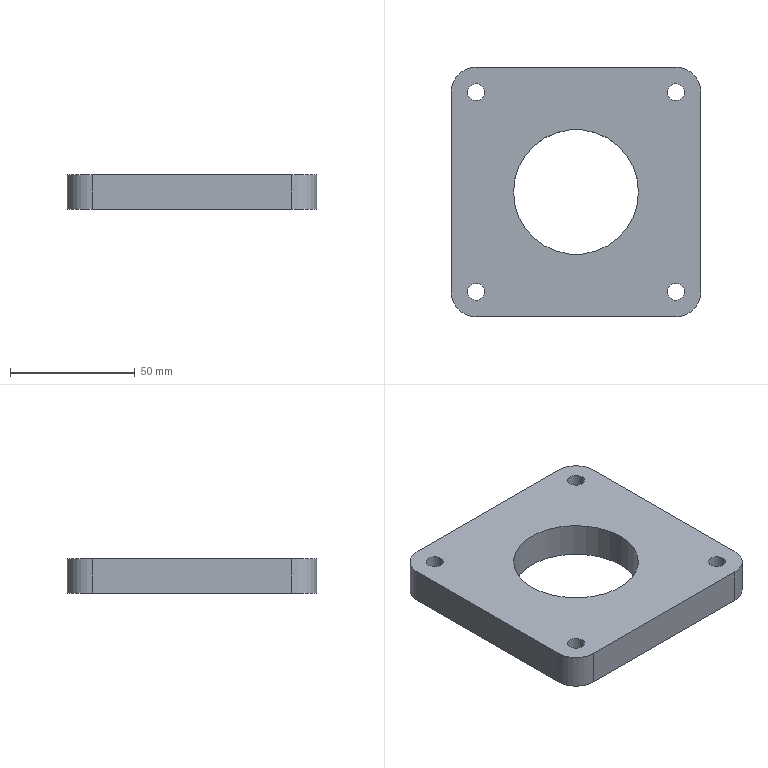Part | SolidWorks | features ICE 2, Extrusion 1, Fillet 1, HoleWzd 1 | 1 solid | 20 faces | box 100 x 100 x 14 mm | volume 109276 mm3 | cylinder 14 | plane 6 | commonest cylinder face diameters 6.8 x8 20 x4 50 x2
STEP:
#1=CARTESIAN_POINT('',(6.6,-10.,0.));
#2=VERTEX_POINT('',#1);
#3=CARTESIAN_POINT('',(13.4,-10.,0.));
#4=VERTEX_POINT('',#3);
#5=CARTESIAN_POINT('',(10.,-10.,0.));
#6=DIRECTION('',(0.,0.,1.));
#7=DIRECTION('',(1.,0.,0.));
#8=AXIS2_PLACEMENT_3D('',#5,#6,#7);
#9=CIRCLE('',#8,3.4);
#10=EDGE_CURVE('',#2,#4,#9,.T.);
#11=ORIENTED_EDGE('',*,*,#10,.F.);
#12=CARTESIAN_POINT('',(6.6,-10.,14.));
#13=VERTEX_POINT('',#12);
#14=CARTESIAN_POINT('',(6.6,-10.,14.));
#15=DIRECTION('',(0.,0.,1.));
#16=VECTOR('',#15,1000.);
#17=LINE('',#14,#16);
#18=EDGE_CURVE('',#2,#13,#17,.T.);
#19=ORIENTED_EDGE('',*,*,#18,.T.);
#20=CARTESIAN_POINT('',(13.4,-10.,14.));
#21=VERTEX_POINT('',#20);
#22=CARTESIAN_POINT('',(10.,-10.,14.));
#23=DIRECTION('',(0.,0.,1.));
#24=DIRECTION('',(1.,0.,0.));
#25=AXIS2_PLACEMENT_3D('',#22,#23,#24);
#26=CIRCLE('',#25,3.4);
#27=EDGE_CURVE('',#13,#21,#26,.T.);
#28=ORIENTED_EDGE('',*,*,#27,.T.);
#29=CARTESIAN_POINT('',(13.4,-10.,14.));
#30=DIRECTION('',(0.,0.,1.));
#31=VECTOR('',#30,1000.);
#32=LINE('',#29,#31);
#33=EDGE_CURVE('',#4,#21,#32,.T.);
#34=ORIENTED_EDGE('',*,*,#33,.F.);
#35=EDGE_LOOP('',(#11,#19,#28,#34));
#36=FACE_OUTER_BOUND('',#35,.T.);
#37=CARTESIAN_POINT('',(10.,-10.,14.));
#38=DIRECTION('',(0.,0.,1.));
#39=DIRECTION('',(1.,0.,0.));
#40=AXIS2_PLACEMENT_3D('',#37,#38,#39);
#41=CYLINDRICAL_SURFACE('',#40,3.4);
#42=ADVANCED_FACE('',(#36),#41,.F.);
#43=CARTESIAN_POINT('',(86.6,-10.,0.));
#44=VERTEX_POINT('',#43);
#45=CARTESIAN_POINT('',(93.4,-10.,0.));
#46=VERTEX_POINT('',#45);
#47=CARTESIAN_POINT('',(90.,-10.,0.));
#48=DIRECTION('',(0.,0.,1.));
#49=DIRECTION('',(1.,0.,0.));
#50=AXIS2_PLACEMENT_3D('',#47,#48,#49);
#51=CIRCLE('',#50,3.4);
#52=EDGE_CURVE('',#44,#46,#51,.T.);
#53=ORIENTED_EDGE('',*,*,#52,.F.);
#54=CARTESIAN_POINT('',(86.6,-10.,14.));
#55=VERTEX_POINT('',#54);
#56=CARTESIAN_POINT('',(86.6,-10.,14.));
#57=DIRECTION('',(0.,0.,1.));
#58=VECTOR('',#57,1000.);
#59=LINE('',#56,#58);
#60=EDGE_CURVE('',#44,#55,#59,.T.);
#61=ORIENTED_EDGE('',*,*,#60,.T.);
#62=CARTESIAN_POINT('',(93.4,-10.,14.));
#63=VERTEX_POINT('',#62);
#64=CARTESIAN_POINT('',(90.,-10.,14.));
#65=DIRECTION('',(0.,0.,1.));
#66=DIRECTION('',(1.,0.,0.));
#67=AXIS2_PLACEMENT_3D('',#64,#65,#66);
#68=CIRCLE('',#67,3.4);
#69=EDGE_CURVE('',#55,#63,#68,.T.);
#70=ORIENTED_EDGE('',*,*,#69,.T.);
#71=CARTESIAN_POINT('',(93.4,-10.,14.));
#72=DIRECTION('',(0.,0.,1.));
#73=VECTOR('',#72,1000.);
#74=LINE('',#71,#73);
#75=EDGE_CURVE('',#46,#63,#74,.T.);
#76=ORIENTED_EDGE('',*,*,#75,.F.);
#77=EDGE_LOOP('',(#53,#61,#70,#76));
#78=FACE_OUTER_BOUND('',#77,.T.);
#79=CARTESIAN_POINT('',(90.,-10.,14.));
#80=DIRECTION('',(0.,0.,1.));
#81=DIRECTION('',(1.,0.,0.));
#82=AXIS2_PLACEMENT_3D('',#79,#80,#81);
#83=CYLINDRICAL_SURFACE('',#82,3.4);
#84=ADVANCED_FACE('',(#78),#83,.F.);
#85=CARTESIAN_POINT('',(6.6,-90.,0.));
#86=VERTEX_POINT('',#85);
#87=CARTESIAN_POINT('',(13.4,-90.,0.));
#88=VERTEX_POINT('',#87);
#89=CARTESIAN_POINT('',(10.,-90.,0.));
#90=DIRECTION('',(0.,0.,1.));
#91=DIRECTION('',(1.,0.,0.));
#92=AXIS2_PLACEMENT_3D('',#89,#90,#91);
#93=CIRCLE('',#92,3.4);
#94=EDGE_CURVE('',#86,#88,#93,.T.);
#95=ORIENTED_EDGE('',*,*,#94,.F.);
#96=CARTESIAN_POINT('',(6.6,-90.,14.));
#97=VERTEX_POINT('',#96);
#98=CARTESIAN_POINT('',(6.6,-90.,14.));
#99=DIRECTION('',(0.,0.,1.));
#100=VECTOR('',#99,1000.);
#101=LINE('',#98,#100);
#102=EDGE_CURVE('',#86,#97,#101,.T.);
#103=ORIENTED_EDGE('',*,*,#102,.T.);
#104=CARTESIAN_POINT('',(13.4,-90.,14.));
#105=VERTEX_POINT('',#104);
#106=CARTESIAN_POINT('',(10.,-90.,14.));
#107=DIRECTION('',(0.,0.,1.));
#108=DIRECTION('',(1.,0.,0.));
#109=AXIS2_PLACEMENT_3D('',#106,#107,#108);
#110=CIRCLE('',#109,3.4);
#111=EDGE_CURVE('',#97,#105,#110,.T.);
#112=ORIENTED_EDGE('',*,*,#111,.T.);
#113=CARTESIAN_POINT('',(13.4,-90.,14.));
#114=DIRECTION('',(0.,0.,1.));
#115=VECTOR('',#114,1000.);
#116=LINE('',#113,#115);
#117=EDGE_CURVE('',#88,#105,#116,.T.);
#118=ORIENTED_EDGE('',*,*,#117,.F.);
#119=EDGE_LOOP('',(#95,#103,#112,#118));
#120=FACE_OUTER_BOUND('',#119,.T.);
#121=CARTESIAN_POINT('',(10.,-90.,14.));
#122=DIRECTION('',(0.,0.,1.));
#123=DIRECTION('',(1.,0.,0.));
#124=AXIS2_PLACEMENT_3D('',#121,#122,#123);
#125=CYLINDRICAL_SURFACE('',#124,3.4);
#126=ADVANCED_FACE('',(#120),#125,.F.);
#127=CARTESIAN_POINT('',(86.6,-90.,0.));
#128=VERTEX_POINT('',#127);
#129=CARTESIAN_POINT('',(93.4,-90.,0.));
#130=VERTEX_POINT('',#129);
#131=CARTESIAN_POINT('',(90.,-90.,0.));
#132=DIRECTION('',(0.,0.,1.));
#133=DIRECTION('',(1.,0.,0.));
#134=AXIS2_PLACEMENT_3D('',#131,#132,#133);
#135=CIRCLE('',#134,3.4);
#136=EDGE_CURVE('',#128,#130,#135,.T.);
#137=ORIENTED_EDGE('',*,*,#136,.F.);
#138=CARTESIAN_POINT('',(86.6,-90.,14.));
#139=VERTEX_POINT('',#138);
#140=CARTESIAN_POINT('',(86.6,-90.,14.));
#141=DIRECTION('',(0.,0.,1.));
#142=VECTOR('',#141,1000.);
#143=LINE('',#140,#142);
#144=EDGE_CURVE('',#128,#139,#143,.T.);
#145=ORIENTED_EDGE('',*,*,#144,.T.);
#146=CARTESIAN_POINT('',(93.4,-90.,14.));
#147=VERTEX_POINT('',#146);
#148=CARTESIAN_POINT('',(90.,-90.,14.));
#149=DIRECTION('',(0.,0.,1.));
#150=DIRECTION('',(1.,0.,0.));
#151=AXIS2_PLACEMENT_3D('',#148,#149,#150);
#152=CIRCLE('',#151,3.4);
#153=EDGE_CURVE('',#139,#147,#152,.T.);
#154=ORIENTED_EDGE('',*,*,#153,.T.);
#155=CARTESIAN_POINT('',(93.4,-90.,14.));
#156=DIRECTION('',(0.,0.,1.));
#157=VECTOR('',#156,1000.);
#158=LINE('',#155,#157);
#159=EDGE_CURVE('',#130,#147,#158,.T.);
#160=ORIENTED_EDGE('',*,*,#159,.F.);
#161=EDGE_LOOP('',(#137,#145,#154,#160));
#162=FACE_OUTER_BOUND('',#161,.T.);
#163=CARTESIAN_POINT('',(90.,-90.,14.));
#164=DIRECTION('',(0.,0.,1.));
#165=DIRECTION('',(1.,0.,0.));
#166=AXIS2_PLACEMENT_3D('',#163,#164,#165);
#167=CYLINDRICAL_SURFACE('',#166,3.4);
#168=ADVANCED_FACE('',(#162),#167,.F.);
#169=CARTESIAN_POINT('',(25.,-50.,0.));
#170=VERTEX_POINT('',#169);
#171=CARTESIAN_POINT('',(75.,-50.,0.));
#172=VERTEX_POINT('',#171);
#173=CARTESIAN_POINT('',(50.,-50.,0.));
#174=DIRECTION('',(0.,0.,1.));
#175=DIRECTION('',(1.,0.,0.));
#176=AXIS2_PLACEMENT_3D('',#173,#174,#175);
#177=CIRCLE('',#176,25.);
#178=EDGE_CURVE('',#170,#172,#177,.T.);
#179=ORIENTED_EDGE('',*,*,#178,.F.);
#180=CARTESIAN_POINT('',(25.,-50.,14.));
#181=VERTEX_POINT('',#180);
#182=CARTESIAN_POINT('',(25.,-50.,0.));
#183=DIRECTION('',(0.,0.,1.));
#184=VECTOR('',#183,1000.);
#185=LINE('',#182,#184);
#186=EDGE_CURVE('',#170,#181,#185,.T.);
#187=ORIENTED_EDGE('',*,*,#186,.T.);
#188=CARTESIAN_POINT('',(75.,-50.,14.));
#189=VERTEX_POINT('',#188);
#190=CARTESIAN_POINT('',(50.,-50.,14.));
#191=DIRECTION('',(0.,0.,1.));
#192=DIRECTION('',(1.,0.,0.));
#193=AXIS2_PLACEMENT_3D('',#190,#191,#192);
#194=CIRCLE('',#193,25.);
#195=EDGE_CURVE('',#181,#189,#194,.T.);
#196=ORIENTED_EDGE('',*,*,#195,.T.);
#197=CARTESIAN_POINT('',(75.,-50.,0.));
#198=DIRECTION('',(0.,0.,1.));
#199=VECTOR('',#198,1000.);
#200=LINE('',#197,#199);
#201=EDGE_CURVE('',#172,#189,#200,.T.);
#202=ORIENTED_EDGE('',*,*,#201,.F.);
#203=EDGE_LOOP('',(#179,#187,#196,#202));
#204=FACE_OUTER_BOUND('',#203,.T.);
#205=CARTESIAN_POINT('',(50.,-50.,0.));
#206=DIRECTION('',(0.,0.,1.));
#207=DIRECTION('',(1.,0.,0.));
#208=AXIS2_PLACEMENT_3D('',#205,#206,#207);
#209=CYLINDRICAL_SURFACE('',#208,25.);
#210=ADVANCED_FACE('',(#204),#209,.F.);
#211=CARTESIAN_POINT('',(0.,-10.,0.));
#212=VERTEX_POINT('',#211);
#213=CARTESIAN_POINT('',(0.,-90.,0.));
#214=VERTEX_POINT('',#213);
#215=CARTESIAN_POINT('',(0.,0.,0.));
#216=DIRECTION('',(0.,-1.,0.));
#217=VECTOR('',#216,1000.);
#218=LINE('',#215,#217);
#219=EDGE_CURVE('',#212,#214,#218,.T.);
#220=ORIENTED_EDGE('',*,*,#219,.T.);
#221=CARTESIAN_POINT('',(0.,-90.,14.));
#222=VERTEX_POINT('',#221);
#223=CARTESIAN_POINT('',(0.,-90.,14.));
#224=DIRECTION('',(0.,0.,1.));
#225=VECTOR('',#224,1000.);
#226=LINE('',#223,#225);
#227=EDGE_CURVE('',#214,#222,#226,.T.);
#228=ORIENTED_EDGE('',*,*,#227,.T.);
#229=CARTESIAN_POINT('',(0.,-10.,14.));
#230=VERTEX_POINT('',#229);
#231=CARTESIAN_POINT('',(0.,0.,14.));
#232=DIRECTION('',(0.,-1.,0.));
#233=VECTOR('',#232,1000.);
#234=LINE('',#231,#233);
#235=EDGE_CURVE('',#230,#222,#234,.T.);
#236=ORIENTED_EDGE('',*,*,#235,.F.);
#237=CARTESIAN_POINT('',(0.,-10.,14.));
#238=DIRECTION('',(0.,0.,-1.));
#239=VECTOR('',#238,1000.);
#240=LINE('',#237,#239);
#241=EDGE_CURVE('',#230,#212,#240,.T.);
#242=ORIENTED_EDGE('',*,*,#241,.T.);
#243=EDGE_LOOP('',(#220,#228,#236,#242));
#244=FACE_OUTER_BOUND('',#243,.T.);
#245=CARTESIAN_POINT('',(0.,0.,14.));
#246=DIRECTION('',(1.,0.,0.));
#247=DIRECTION('',(0.,1.,0.));
#248=AXIS2_PLACEMENT_3D('',#245,#246,#247);
#249=PLANE('',#248);
#250=ADVANCED_FACE('',(#244),#249,.F.);
#251=CARTESIAN_POINT('',(10.,-100.,14.));
#252=VERTEX_POINT('',#251);
#253=CARTESIAN_POINT('',(90.,-100.,14.));
#254=VERTEX_POINT('',#253);
#255=CARTESIAN_POINT('',(0.,-100.,14.));
#256=DIRECTION('',(1.,0.,0.));
#257=VECTOR('',#256,1000.);
#258=LINE('',#255,#257);
#259=EDGE_CURVE('',#252,#254,#258,.T.);
#260=ORIENTED_EDGE('',*,*,#259,.F.);
#261=CARTESIAN_POINT('',(10.,-100.,0.));
#262=VERTEX_POINT('',#261);
#263=CARTESIAN_POINT('',(10.,-100.,14.));
#264=DIRECTION('',(0.,0.,-1.));
#265=VECTOR('',#264,1000.);
#266=LINE('',#263,#265);
#267=EDGE_CURVE('',#252,#262,#266,.T.);
#268=ORIENTED_EDGE('',*,*,#267,.T.);
#269=CARTESIAN_POINT('',(90.,-100.,0.));
#270=VERTEX_POINT('',#269);
#271=CARTESIAN_POINT('',(0.,-100.,0.));
#272=DIRECTION('',(1.,0.,0.));
#273=VECTOR('',#272,1000.);
#274=LINE('',#271,#273);
#275=EDGE_CURVE('',#262,#270,#274,.T.);
#276=ORIENTED_EDGE('',*,*,#275,.T.);
#277=CARTESIAN_POINT('',(90.,-100.,14.));
#278=DIRECTION('',(0.,0.,1.));
#279=VECTOR('',#278,1000.);
#280=LINE('',#277,#279);
#281=EDGE_CURVE('',#270,#254,#280,.T.);
#282=ORIENTED_EDGE('',*,*,#281,.T.);
#283=EDGE_LOOP('',(#260,#268,#276,#282));
#284=FACE_OUTER_BOUND('',#283,.T.);
#285=CARTESIAN_POINT('',(0.,-100.,14.));
#286=DIRECTION('',(0.,1.,0.));
#287=DIRECTION('',(0.,0.,1.));
#288=AXIS2_PLACEMENT_3D('',#285,#286,#287);
#289=PLANE('',#288);
#290=ADVANCED_FACE('',(#284),#289,.F.);
#291=CARTESIAN_POINT('',(100.,-90.,14.));
#292=VERTEX_POINT('',#291);
#293=CARTESIAN_POINT('',(100.,-10.,14.));
#294=VERTEX_POINT('',#293);
#295=CARTESIAN_POINT('',(100.,0.,14.));
#296=DIRECTION('',(0.,1.,0.));
#297=VECTOR('',#296,1000.);
#298=LINE('',#295,#297);
#299=EDGE_CURVE('',#292,#294,#298,.T.);
#300=ORIENTED_EDGE('',*,*,#299,.F.);
#301=CARTESIAN_POINT('',(100.,-90.,0.));
#302=VERTEX_POINT('',#301);
#303=CARTESIAN_POINT('',(100.,-90.,14.));
#304=DIRECTION('',(0.,0.,-1.));
#305=VECTOR('',#304,1000.);
#306=LINE('',#303,#305);
#307=EDGE_CURVE('',#292,#302,#306,.T.);
#308=ORIENTED_EDGE('',*,*,#307,.T.);
#309=CARTESIAN_POINT('',(100.,-10.,0.));
#310=VERTEX_POINT('',#309);
#311=CARTESIAN_POINT('',(100.,0.,0.));
#312=DIRECTION('',(0.,1.,0.));
#313=VECTOR('',#312,1000.);
#314=LINE('',#311,#313);
#315=EDGE_CURVE('',#302,#310,#314,.T.);
#316=ORIENTED_EDGE('',*,*,#315,.T.);
#317=CARTESIAN_POINT('',(100.,-10.,14.));
#318=DIRECTION('',(0.,0.,1.));
#319=VECTOR('',#318,1000.);
#320=LINE('',#317,#319);
#321=EDGE_CURVE('',#310,#294,#320,.T.);
#322=ORIENTED_EDGE('',*,*,#321,.T.);
#323=EDGE_LOOP('',(#300,#308,#316,#322));
#324=FACE_OUTER_BOUND('',#323,.T.);
#325=CARTESIAN_POINT('',(100.,0.,14.));
#326=DIRECTION('',(-1.,0.,0.));
#327=DIRECTION('',(0.,-1.,0.));
#328=AXIS2_PLACEMENT_3D('',#325,#326,#327);
#329=PLANE('',#328);
#330=ADVANCED_FACE('',(#324),#329,.F.);
#331=CARTESIAN_POINT('',(90.,0.,14.));
#332=VERTEX_POINT('',#331);
#333=CARTESIAN_POINT('',(10.,0.,14.));
#334=VERTEX_POINT('',#333);
#335=CARTESIAN_POINT('',(0.,0.,14.));
#336=DIRECTION('',(-1.,0.,0.));
#337=VECTOR('',#336,1000.);
#338=LINE('',#335,#337);
#339=EDGE_CURVE('',#332,#334,#338,.T.);
#340=ORIENTED_EDGE('',*,*,#339,.F.);
#341=CARTESIAN_POINT('',(90.,0.,0.));
#342=VERTEX_POINT('',#341);
#343=CARTESIAN_POINT('',(90.,0.,14.));
#344=DIRECTION('',(0.,0.,-1.));
#345=VECTOR('',#344,1000.);
#346=LINE('',#343,#345);
#347=EDGE_CURVE('',#332,#342,#346,.T.);
#348=ORIENTED_EDGE('',*,*,#347,.T.);
#349=CARTESIAN_POINT('',(10.,0.,0.));
#350=VERTEX_POINT('',#349);
#351=CARTESIAN_POINT('',(0.,0.,0.));
#352=DIRECTION('',(-1.,0.,0.));
#353=VECTOR('',#352,1000.);
#354=LINE('',#351,#353);
#355=EDGE_CURVE('',#342,#350,#354,.T.);
#356=ORIENTED_EDGE('',*,*,#355,.T.);
#357=CARTESIAN_POINT('',(10.,0.,14.));
#358=DIRECTION('',(0.,0.,1.));
#359=VECTOR('',#358,1000.);
#360=LINE('',#357,#359);
#361=EDGE_CURVE('',#350,#334,#360,.T.);
#362=ORIENTED_EDGE('',*,*,#361,.T.);
#363=EDGE_LOOP('',(#340,#348,#356,#362));
#364=FACE_OUTER_BOUND('',#363,.T.);
#365=CARTESIAN_POINT('',(0.,0.,14.));
#366=DIRECTION('',(0.,-1.,0.));
#367=DIRECTION('',(0.,0.,-1.));
#368=AXIS2_PLACEMENT_3D('',#365,#366,#367);
#369=PLANE('',#368);
#370=ADVANCED_FACE('',(#364),#369,.F.);
#371=CARTESIAN_POINT('',(10.,-10.,14.));
#372=DIRECTION('',(0.,0.,1.));
#373=DIRECTION('',(1.,0.,0.));
#374=AXIS2_PLACEMENT_3D('',#371,#372,#373);
#375=CIRCLE('',#374,3.4);
#376=EDGE_CURVE('',#21,#13,#375,.T.);
#377=ORIENTED_EDGE('',*,*,#376,.F.);
#378=ORIENTED_EDGE('',*,*,#27,.F.);
#379=EDGE_LOOP('',(#377,#378));
#380=FACE_BOUND('',#379,.T.);
#381=CARTESIAN_POINT('',(90.,-10.,14.));
#382=DIRECTION('',(0.,0.,1.));
#383=DIRECTION('',(1.,0.,0.));
#384=AXIS2_PLACEMENT_3D('',#381,#382,#383);
#385=CIRCLE('',#384,3.4);
#386=EDGE_CURVE('',#63,#55,#385,.T.);
#387=ORIENTED_EDGE('',*,*,#386,.F.);
#388=ORIENTED_EDGE('',*,*,#69,.F.);
#389=EDGE_LOOP('',(#387,#388));
#390=FACE_BOUND('',#389,.T.);
#391=CARTESIAN_POINT('',(10.,-90.,14.));
#392=DIRECTION('',(0.,0.,1.));
#393=DIRECTION('',(1.,0.,0.));
#394=AXIS2_PLACEMENT_3D('',#391,#392,#393);
#395=CIRCLE('',#394,3.4);
#396=EDGE_CURVE('',#105,#97,#395,.T.);
#397=ORIENTED_EDGE('',*,*,#396,.F.);
#398=ORIENTED_EDGE('',*,*,#111,.F.);
#399=EDGE_LOOP('',(#397,#398));
#400=FACE_BOUND('',#399,.T.);
#401=CARTESIAN_POINT('',(90.,-90.,14.));
#402=DIRECTION('',(0.,0.,1.));
#403=DIRECTION('',(1.,0.,0.));
#404=AXIS2_PLACEMENT_3D('',#401,#402,#403);
#405=CIRCLE('',#404,3.4);
#406=EDGE_CURVE('',#147,#139,#405,.T.);
#407=ORIENTED_EDGE('',*,*,#406,.F.);
#408=ORIENTED_EDGE('',*,*,#153,.F.);
#409=EDGE_LOOP('',(#407,#408));
#410=FACE_BOUND('',#409,.T.);
#411=CARTESIAN_POINT('',(50.,-50.,14.));
#412=DIRECTION('',(0.,0.,1.));
#413=DIRECTION('',(1.,0.,0.));
#414=AXIS2_PLACEMENT_3D('',#411,#412,#413);
#415=CIRCLE('',#414,25.);
#416=EDGE_CURVE('',#189,#181,#415,.T.);
#417=ORIENTED_EDGE('',*,*,#416,.F.);
#418=ORIENTED_EDGE('',*,*,#195,.F.);
#419=EDGE_LOOP('',(#417,#418));
#420=FACE_BOUND('',#419,.T.);
#421=ORIENTED_EDGE('',*,*,#235,.T.);
#422=CARTESIAN_POINT('',(10.,-90.,14.));
#423=DIRECTION('',(0.,0.,1.));
#424=DIRECTION('',(1.,0.,0.));
#425=AXIS2_PLACEMENT_3D('',#422,#423,#424);
#426=CIRCLE('',#425,10.);
#427=EDGE_CURVE('',#222,#252,#426,.T.);
#428=ORIENTED_EDGE('',*,*,#427,.T.);
#429=ORIENTED_EDGE('',*,*,#259,.T.);
#430=CARTESIAN_POINT('',(90.,-90.,14.));
#431=DIRECTION('',(0.,0.,1.));
#432=DIRECTION('',(1.,0.,0.));
#433=AXIS2_PLACEMENT_3D('',#430,#431,#432);
#434=CIRCLE('',#433,10.);
#435=EDGE_CURVE('',#254,#292,#434,.T.);
#436=ORIENTED_EDGE('',*,*,#435,.T.);
#437=ORIENTED_EDGE('',*,*,#299,.T.);
#438=CARTESIAN_POINT('',(90.,-10.,14.));
#439=DIRECTION('',(0.,0.,1.));
#440=DIRECTION('',(1.,0.,0.));
#441=AXIS2_PLACEMENT_3D('',#438,#439,#440);
#442=CIRCLE('',#441,10.);
#443=EDGE_CURVE('',#294,#332,#442,.T.);
#444=ORIENTED_EDGE('',*,*,#443,.T.);
#445=ORIENTED_EDGE('',*,*,#339,.T.);
#446=CARTESIAN_POINT('',(10.,-10.,14.));
#447=DIRECTION('',(0.,0.,1.));
#448=DIRECTION('',(1.,0.,0.));
#449=AXIS2_PLACEMENT_3D('',#446,#447,#448);
#450=CIRCLE('',#449,10.);
#451=EDGE_CURVE('',#334,#230,#450,.T.);
#452=ORIENTED_EDGE('',*,*,#451,.T.);
#453=EDGE_LOOP('',(#421,#428,#429,#436,#437,#444,#445,#452));
#454=FACE_OUTER_BOUND('',#453,.T.);
#455=CARTESIAN_POINT('',(0.,0.,14.));
#456=DIRECTION('',(0.,0.,1.));
#457=DIRECTION('',(1.,0.,0.));
#458=AXIS2_PLACEMENT_3D('',#455,#456,#457);
#459=PLANE('',#458);
#460=ADVANCED_FACE('',(#380,#390,#400,#410,#420,#454),#459,.T.);
#461=CARTESIAN_POINT('',(10.,-10.,0.));
#462=DIRECTION('',(0.,0.,1.));
#463=DIRECTION('',(1.,0.,0.));
#464=AXIS2_PLACEMENT_3D('',#461,#462,#463);
#465=CIRCLE('',#464,3.4);
#466=EDGE_CURVE('',#4,#2,#465,.T.);
#467=ORIENTED_EDGE('',*,*,#466,.T.);
#468=ORIENTED_EDGE('',*,*,#10,.T.);
#469=EDGE_LOOP('',(#467,#468));
#470=FACE_BOUND('',#469,.T.);
#471=CARTESIAN_POINT('',(90.,-10.,0.));
#472=DIRECTION('',(0.,0.,1.));
#473=DIRECTION('',(1.,0.,0.));
#474=AXIS2_PLACEMENT_3D('',#471,#472,#473);
#475=CIRCLE('',#474,3.4);
#476=EDGE_CURVE('',#46,#44,#475,.T.);
#477=ORIENTED_EDGE('',*,*,#476,.T.);
#478=ORIENTED_EDGE('',*,*,#52,.T.);
#479=EDGE_LOOP('',(#477,#478));
#480=FACE_BOUND('',#479,.T.);
#481=CARTESIAN_POINT('',(10.,-90.,0.));
#482=DIRECTION('',(0.,0.,1.));
#483=DIRECTION('',(1.,0.,0.));
#484=AXIS2_PLACEMENT_3D('',#481,#482,#483);
#485=CIRCLE('',#484,3.4);
#486=EDGE_CURVE('',#88,#86,#485,.T.);
#487=ORIENTED_EDGE('',*,*,#486,.T.);
#488=ORIENTED_EDGE('',*,*,#94,.T.);
#489=EDGE_LOOP('',(#487,#488));
#490=FACE_BOUND('',#489,.T.);
#491=CARTESIAN_POINT('',(90.,-90.,0.));
#492=DIRECTION('',(0.,0.,1.));
#493=DIRECTION('',(1.,0.,0.));
#494=AXIS2_PLACEMENT_3D('',#491,#492,#493);
#495=CIRCLE('',#494,3.4);
#496=EDGE_CURVE('',#130,#128,#495,.T.);
#497=ORIENTED_EDGE('',*,*,#496,.T.);
#498=ORIENTED_EDGE('',*,*,#136,.T.);
#499=EDGE_LOOP('',(#497,#498));
#500=FACE_BOUND('',#499,.T.);
#501=CARTESIAN_POINT('',(50.,-50.,0.));
#502=DIRECTION('',(0.,0.,1.));
#503=DIRECTION('',(1.,0.,0.));
#504=AXIS2_PLACEMENT_3D('',#501,#502,#503);
#505=CIRCLE('',#504,25.);
#506=EDGE_CURVE('',#172,#170,#505,.T.);
#507=ORIENTED_EDGE('',*,*,#506,.T.);
#508=ORIENTED_EDGE('',*,*,#178,.T.);
#509=EDGE_LOOP('',(#507,#508));
#510=FACE_BOUND('',#509,.T.);
#511=ORIENTED_EDGE('',*,*,#275,.F.);
#512=CARTESIAN_POINT('',(10.,-90.,0.));
#513=DIRECTION('',(0.,0.,-1.));
#514=DIRECTION('',(1.,0.,0.));
#515=AXIS2_PLACEMENT_3D('',#512,#513,#514);
#516=CIRCLE('',#515,10.);
#517=EDGE_CURVE('',#262,#214,#516,.T.);
#518=ORIENTED_EDGE('',*,*,#517,.T.);
#519=ORIENTED_EDGE('',*,*,#219,.F.);
#520=CARTESIAN_POINT('',(10.,-10.,0.));
#521=DIRECTION('',(0.,0.,-1.));
#522=DIRECTION('',(1.,0.,0.));
#523=AXIS2_PLACEMENT_3D('',#520,#521,#522);
#524=CIRCLE('',#523,10.);
#525=EDGE_CURVE('',#212,#350,#524,.T.);
#526=ORIENTED_EDGE('',*,*,#525,.T.);
#527=ORIENTED_EDGE('',*,*,#355,.F.);
#528=CARTESIAN_POINT('',(90.,-10.,0.));
#529=DIRECTION('',(0.,0.,-1.));
#530=DIRECTION('',(1.,0.,0.));
#531=AXIS2_PLACEMENT_3D('',#528,#529,#530);
#532=CIRCLE('',#531,10.);
#533=EDGE_CURVE('',#342,#310,#532,.T.);
#534=ORIENTED_EDGE('',*,*,#533,.T.);
#535=ORIENTED_EDGE('',*,*,#315,.F.);
#536=CARTESIAN_POINT('',(90.,-90.,0.));
#537=DIRECTION('',(0.,0.,-1.));
#538=DIRECTION('',(1.,0.,0.));
#539=AXIS2_PLACEMENT_3D('',#536,#537,#538);
#540=CIRCLE('',#539,10.);
#541=EDGE_CURVE('',#302,#270,#540,.T.);
#542=ORIENTED_EDGE('',*,*,#541,.T.);
#543=EDGE_LOOP('',(#511,#518,#519,#526,#527,#534,#535,#542));
#544=FACE_OUTER_BOUND('',#543,.T.);
#545=CARTESIAN_POINT('',(0.,0.,0.));
#546=DIRECTION('',(0.,0.,1.));
#547=DIRECTION('',(1.,0.,0.));
#548=AXIS2_PLACEMENT_3D('',#545,#546,#547);
#549=PLANE('',#548);
#550=ADVANCED_FACE('',(#470,#480,#490,#500,#510,#544),#549,.F.);
#551=ORIENTED_EDGE('',*,*,#186,.F.);
#552=ORIENTED_EDGE('',*,*,#506,.F.);
#553=ORIENTED_EDGE('',*,*,#201,.T.);
#554=ORIENTED_EDGE('',*,*,#416,.T.);
#555=EDGE_LOOP('',(#551,#552,#553,#554));
#556=FACE_OUTER_BOUND('',#555,.T.);
#557=CARTESIAN_POINT('',(50.,-50.,0.));
#558=DIRECTION('',(0.,0.,1.));
#559=DIRECTION('',(1.,0.,0.));
#560=AXIS2_PLACEMENT_3D('',#557,#558,#559);
#561=CYLINDRICAL_SURFACE('',#560,25.);
#562=ADVANCED_FACE('',(#556),#561,.F.);
#563=ORIENTED_EDGE('',*,*,#144,.F.);
#564=ORIENTED_EDGE('',*,*,#496,.F.);
#565=ORIENTED_EDGE('',*,*,#159,.T.);
#566=ORIENTED_EDGE('',*,*,#406,.T.);
#567=EDGE_LOOP('',(#563,#564,#565,#566));
#568=FACE_OUTER_BOUND('',#567,.T.);
#569=CARTESIAN_POINT('',(90.,-90.,14.));
#570=DIRECTION('',(0.,0.,1.));
#571=DIRECTION('',(1.,0.,0.));
#572=AXIS2_PLACEMENT_3D('',#569,#570,#571);
#573=CYLINDRICAL_SURFACE('',#572,3.4);
#574=ADVANCED_FACE('',(#568),#573,.F.);
#575=ORIENTED_EDGE('',*,*,#102,.F.);
#576=ORIENTED_EDGE('',*,*,#486,.F.);
#577=ORIENTED_EDGE('',*,*,#117,.T.);
#578=ORIENTED_EDGE('',*,*,#396,.T.);
#579=EDGE_LOOP('',(#575,#576,#577,#578));
#580=FACE_OUTER_BOUND('',#579,.T.);
#581=CARTESIAN_POINT('',(10.,-90.,14.));
#582=DIRECTION('',(0.,0.,1.));
#583=DIRECTION('',(1.,0.,0.));
#584=AXIS2_PLACEMENT_3D('',#581,#582,#583);
#585=CYLINDRICAL_SURFACE('',#584,3.4);
#586=ADVANCED_FACE('',(#580),#585,.F.);
#587=ORIENTED_EDGE('',*,*,#60,.F.);
#588=ORIENTED_EDGE('',*,*,#476,.F.);
#589=ORIENTED_EDGE('',*,*,#75,.T.);
#590=ORIENTED_EDGE('',*,*,#386,.T.);
#591=EDGE_LOOP('',(#587,#588,#589,#590));
#592=FACE_OUTER_BOUND('',#591,.T.);
#593=CARTESIAN_POINT('',(90.,-10.,14.));
#594=DIRECTION('',(0.,0.,1.));
#595=DIRECTION('',(1.,0.,0.));
#596=AXIS2_PLACEMENT_3D('',#593,#594,#595);
#597=CYLINDRICAL_SURFACE('',#596,3.4);
#598=ADVANCED_FACE('',(#592),#597,.F.);
#599=ORIENTED_EDGE('',*,*,#18,.F.);
#600=ORIENTED_EDGE('',*,*,#466,.F.);
#601=ORIENTED_EDGE('',*,*,#33,.T.);
#602=ORIENTED_EDGE('',*,*,#376,.T.);
#603=EDGE_LOOP('',(#599,#600,#601,#602));
#604=FACE_OUTER_BOUND('',#603,.T.);
#605=CARTESIAN_POINT('',(10.,-10.,14.));
#606=DIRECTION('',(0.,0.,1.));
#607=DIRECTION('',(1.,0.,0.));
#608=AXIS2_PLACEMENT_3D('',#605,#606,#607);
#609=CYLINDRICAL_SURFACE('',#608,3.4);
#610=ADVANCED_FACE('',(#604),#609,.F.);
#611=ORIENTED_EDGE('',*,*,#427,.F.);
#612=ORIENTED_EDGE('',*,*,#227,.F.);
#613=ORIENTED_EDGE('',*,*,#517,.F.);
#614=ORIENTED_EDGE('',*,*,#267,.F.);
#615=EDGE_LOOP('',(#611,#612,#613,#614));
#616=FACE_OUTER_BOUND('',#615,.T.);
#617=CARTESIAN_POINT('',(10.,-90.,14.));
#618=DIRECTION('',(0.,0.,-1.));
#619=DIRECTION('',(-1.,0.,0.));
#620=AXIS2_PLACEMENT_3D('',#617,#618,#619);
#621=CYLINDRICAL_SURFACE('',#620,10.);
#622=ADVANCED_FACE('',(#616),#621,.T.);
#623=ORIENTED_EDGE('',*,*,#435,.F.);
#624=ORIENTED_EDGE('',*,*,#281,.F.);
#625=ORIENTED_EDGE('',*,*,#541,.F.);
#626=ORIENTED_EDGE('',*,*,#307,.F.);
#627=EDGE_LOOP('',(#623,#624,#625,#626));
#628=FACE_OUTER_BOUND('',#627,.T.);
#629=CARTESIAN_POINT('',(90.,-90.,14.));
#630=DIRECTION('',(0.,0.,-1.));
#631=DIRECTION('',(-1.,0.,0.));
#632=AXIS2_PLACEMENT_3D('',#629,#630,#631);
#633=CYLINDRICAL_SURFACE('',#632,10.);
#634=ADVANCED_FACE('',(#628),#633,.T.);
#635=ORIENTED_EDGE('',*,*,#443,.F.);
#636=ORIENTED_EDGE('',*,*,#321,.F.);
#637=ORIENTED_EDGE('',*,*,#533,.F.);
#638=ORIENTED_EDGE('',*,*,#347,.F.);
#639=EDGE_LOOP('',(#635,#636,#637,#638));
#640=FACE_OUTER_BOUND('',#639,.T.);
#641=CARTESIAN_POINT('',(90.,-10.,14.));
#642=DIRECTION('',(0.,0.,-1.));
#643=DIRECTION('',(-1.,0.,0.));
#644=AXIS2_PLACEMENT_3D('',#641,#642,#643);
#645=CYLINDRICAL_SURFACE('',#644,10.);
#646=ADVANCED_FACE('',(#640),#645,.T.);
#647=ORIENTED_EDGE('',*,*,#451,.F.);
#648=ORIENTED_EDGE('',*,*,#361,.F.);
#649=ORIENTED_EDGE('',*,*,#525,.F.);
#650=ORIENTED_EDGE('',*,*,#241,.F.);
#651=EDGE_LOOP('',(#647,#648,#649,#650));
#652=FACE_OUTER_BOUND('',#651,.T.);
#653=CARTESIAN_POINT('',(10.,-10.,14.));
#654=DIRECTION('',(0.,0.,-1.));
#655=DIRECTION('',(-1.,0.,0.));
#656=AXIS2_PLACEMENT_3D('',#653,#654,#655);
#657=CYLINDRICAL_SURFACE('',#656,10.);
#658=ADVANCED_FACE('',(#652),#657,.T.);
#659=CLOSED_SHELL('',(#42,#84,#126,#168,#210,#250,#290,#330,#370,#460,#550,#562,#574,#586,#598,#610,#622,#634,#646,#658));
#660=MANIFOLD_SOLID_BREP('',#659);
#661=CARTESIAN_POINT('',(0.,0.,0.));
#662=DIRECTION('',(0.,0.,1.));
#663=DIRECTION('',(1.,0.,0.));
#664=AXIS2_PLACEMENT_3D('',#661,#662,#663);
#665=(LENGTH_UNIT()NAMED_UNIT(*)SI_UNIT(.MILLI.,.METRE.));
#666=UNCERTAINTY_MEASURE_WITH_UNIT(LENGTH_MEASURE(0.00001),#665,'','');
#667=(NAMED_UNIT(*)PLANE_ANGLE_UNIT()SI_UNIT($,.RADIAN.));
#668=(NAMED_UNIT(*)SI_UNIT($,.STERADIAN.)SOLID_ANGLE_UNIT());
#669=(GEOMETRIC_REPRESENTATION_CONTEXT(3)GLOBAL_UNCERTAINTY_ASSIGNED_CONTEXT((#666))GLOBAL_UNIT_ASSIGNED_CONTEXT((#665,#667,#668))REPRESENTATION_CONTEXT('',''));
#670=ADVANCED_BREP_SHAPE_REPRESENTATION('',(#660,#664),#669);